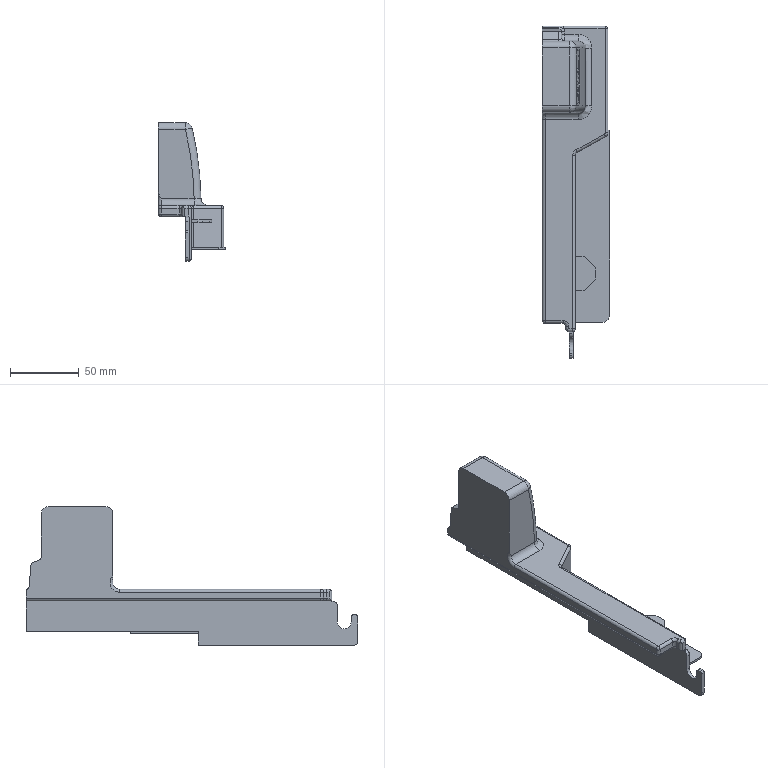Part | STEP file | DEWALT-DWE7492-B2_002 | 1 solid | 175 faces | box 48.75 x 241 x 100.5 mm | volume 225143 mm3 | plane 94 | cylinder 46 | spline 21 | torus 7 | sphere 6 | other 1 | commonest cylinder face diameters 4 x23 10 x12 6 x6 1 x2 3 x2 487.5 x1